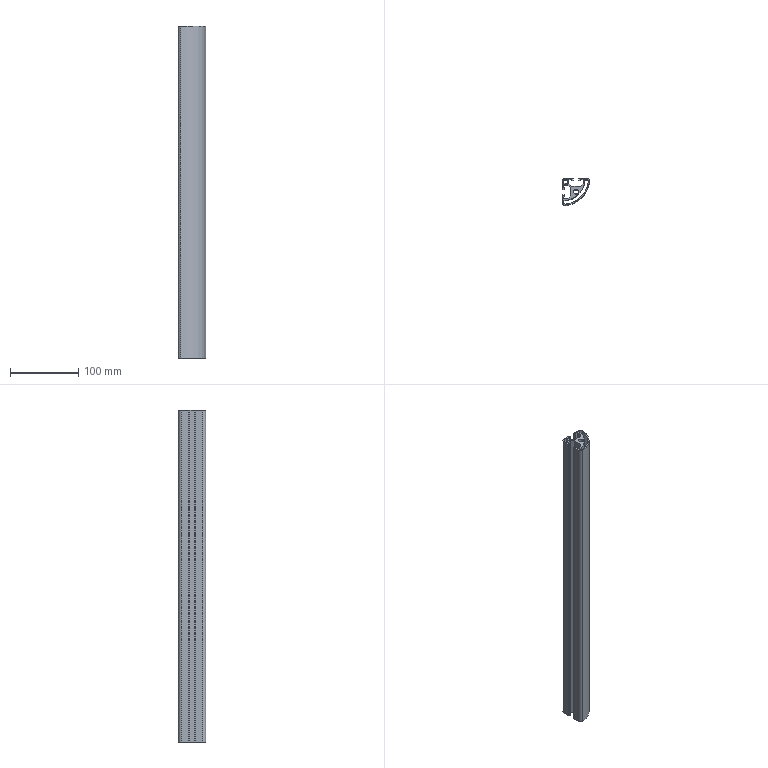Part | 1 solid | 59 faces | box 39.857 x 39.857 x 485 mm | volume 236527 mm3 | plane 48 | cylinder 11 | commonest cylinder face diameters 5 x3 9 x3 6.8 x2 66.41 x1 76.531 x1 80 x1